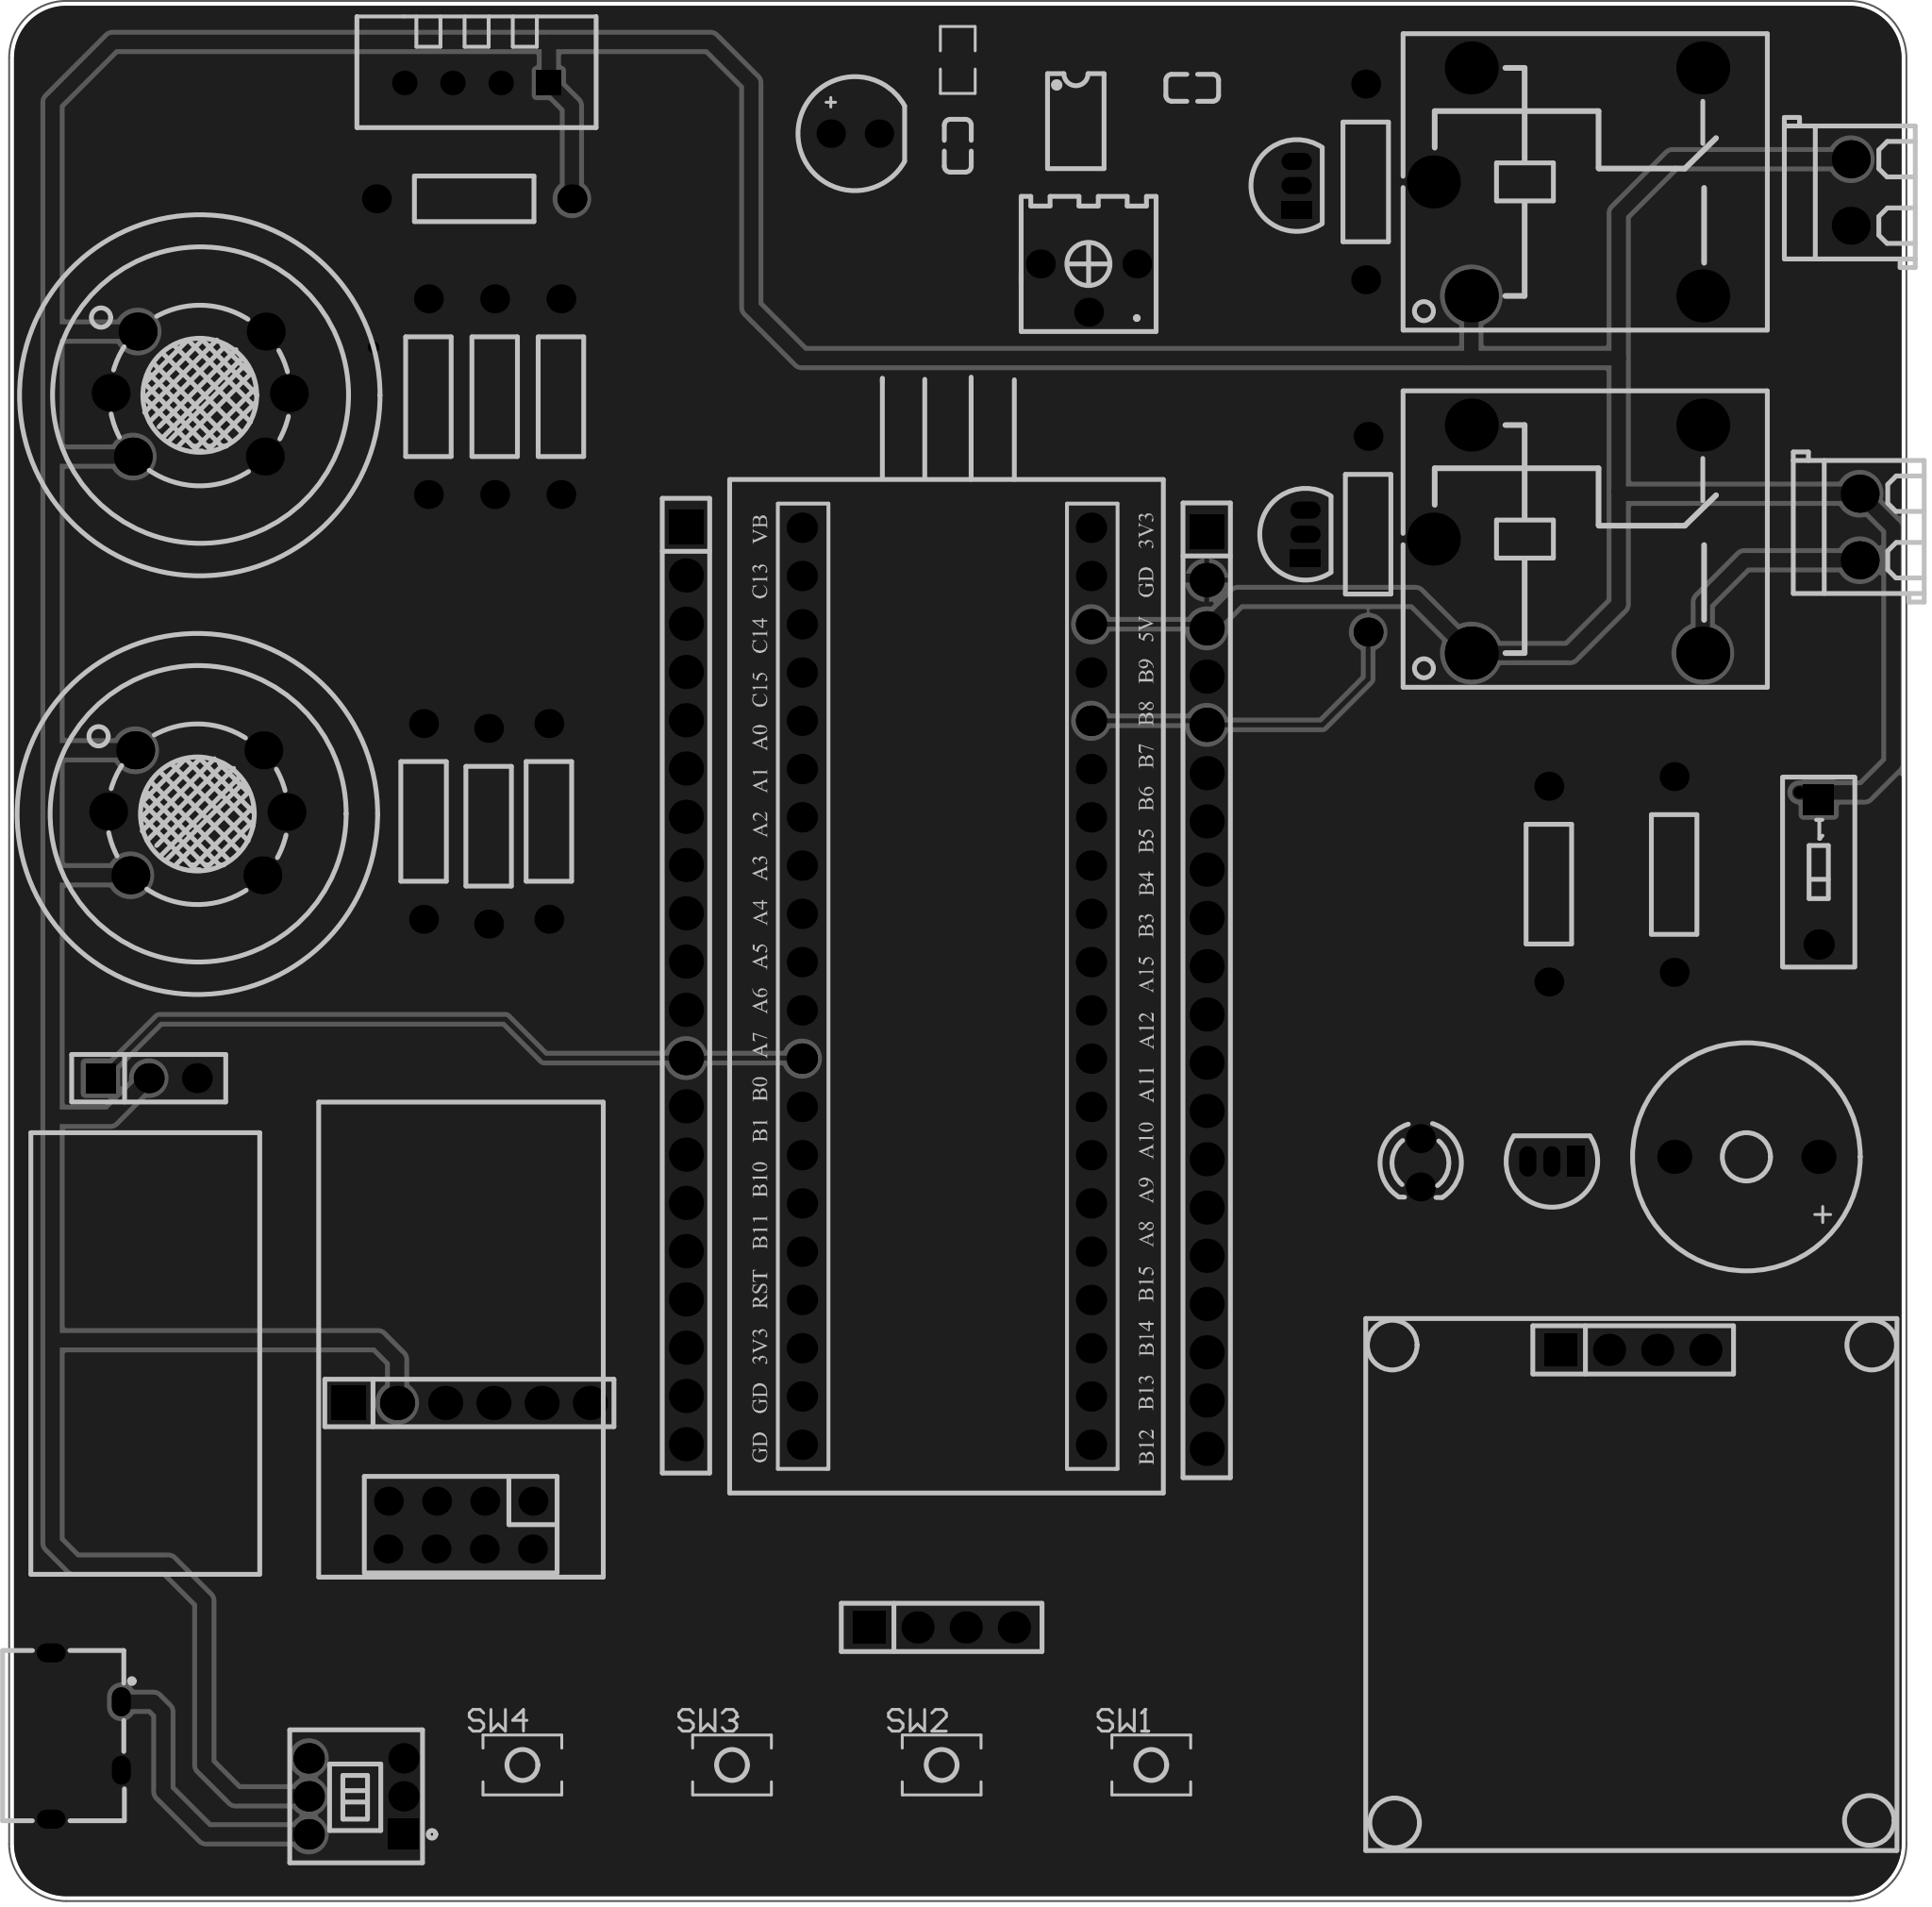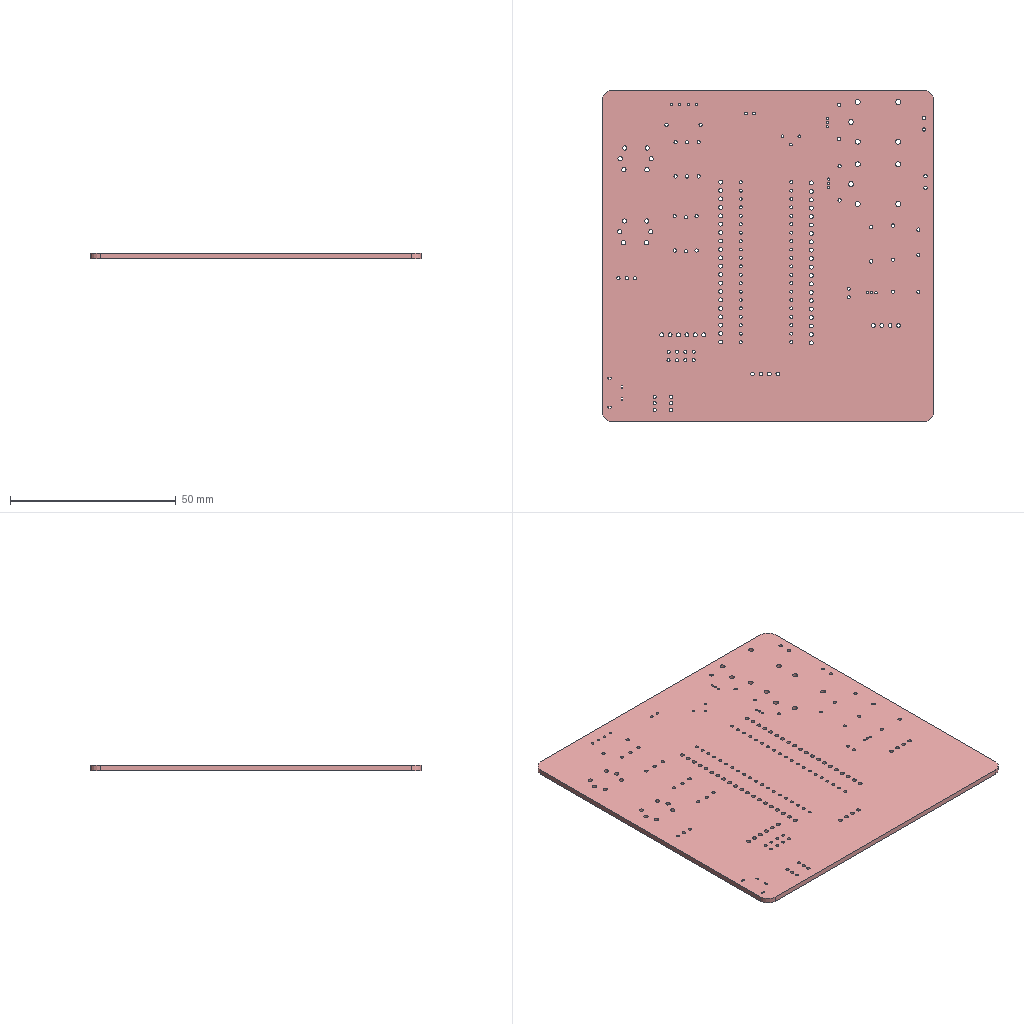Circuit board layout | Altium Designer | box 100 x 100 x 1.6 mm
Layer stack:
# Altium Designer layer stack of  (unit mm; dielectric type: 0 none, 1 core, 2 prepreg, 3 surface material)
index,name,kind,layer,copper_thickness_mm,dielectric_type,dielectric_thickness_mm,dielectric_material,dielectric_constant
0,Top Paste Mask Layer,other,,,,,,
1,Top Silkscreen Layer,other,,,,,,
2,Top Solder Mask Layer,dielectric,,,3,0.01,,3.3
3,Top Layer,copper,Top Layer,0.035,,,,
4,Dielectric1,dielectric,,,3,1.51,FR4,4.5
5,Bottom Layer,copper,Bottom Layer,0.035,,,,
6,Bottom Solder Mask Layer,dielectric,,,3,0.01,,3.3
7,Bottom Silkscreen Layer,other,,,,,,
8,Bottom Paste Mask Layer,other,,,,,,
# drill layer pairs: low layer,high layer
drill_pair,Top Layer,Bottom Layer
Part placement:
Designator,Comment,Layer,Footprint,Center-X(mm),Center-Y(mm),Rotation
H3,,TopLayer,HDR-TH_20P-P2.54-V-F,146.812,132.588,270
H4,,TopLayer,HDR-TH_20P-P2.54-V-F,119.366,132.831,270
H6,,TopLayer,HDR-TH_3P-P2.54-V-F,91.048,127.962,0
H7,,TopLayer,HDR-TH_4P-P2.54-V-F,132.842,99.06,0
SW5,NDS-01V,TopLayer,SW-TH_2P-L3.9-W9.9-P2.54-LS7.6,179.07,138.811,270
U1,MQ-2,TopLayer,SENSOR-TH_MQ-2,93.614,141.932,0
U7,DHT11,TopLayer,SENSOR-TH_DHT11,108.331,180.34,180
BUZZER1,2.3kHz,TopLayer,BUZ-TH_BD12.0-P7.60-D0.6-FD,175.26,123.825,180
H10,2.54-1*4P female,TopLayer,HDR-TH_4P-P2.54-V-F,169.291,113.665,0
H13,,TopLayer,HDR-TH_6P-P2.54-V-M-1,107.95,110.871,0
Q1,,TopLayer,S8050_TO_92,165.006,123.586,180
R8,1kΩ,TopLayer,Res_1/4W,171.45,138.684,270
R9,120,TopLayer,Res_1/4W,164.846,138.176,270
SW8,TK-6700-1,TopLayer,SW-TH_TK-6700-1,101.981,90.17,90
U2,MQ-5,TopLayer,SENSOR-TH_MQ-2,93.741,163.967,0
U44,,TopLayer,STM32最小系统板,133.098,132.803,0
U98,,TopLayer,WiFi封装,107.479,104.445,0
USB1,KH-TYPE-C-2P,TopLayer,USB-SMD_KH-TYPE-C-2P,87.757,93.345,270
Q2,,TopLayer,S8050_TO_92,151.556,174.944,90
R1,10kΩ,TopLayer,Res_1/4W,108.966,141.224,90
R2,10kΩ,TopLayer,Res_1/4W,112.141,141.478,90
R3,5Ω,TopLayer,Res_1/4W,105.537,141.478,90
R4,10kΩ,TopLayer,Res_1/4W,109.284,163.83,90
R5,10kΩ,TopLayer,Res_1/4W,112.776,163.83,90
R6,5Ω,TopLayer,Res_1/4W,105.791,163.83,90
R13,10kΩ,TopLayer,Res_1/4W,108.204,174.244,0
R15,1kΩ,TopLayer,Res_1/4W,155.194,175.133,90
RLY1,SRD-05VDC-SL-C,TopLayer,RELAY-TH_SRD-XXVDC-XL-C,165.862,175.133,0
U4,KF350-3.5-2P,TopLayer,CONN-TH_P3.50_KF350-3.5-2P,180.759,174.577,90
Q3,,TopLayer,S8050_TO_92,152.019,156.591,90
R10,1kΩ,TopLayer,Res_1/4W,155.321,156.591,90
RLY2,SRD-05VDC-SL-C,TopLayer,RELAY-TH_SRD-XXVDC-XL-C,165.862,156.337,0
U5,KF350-3.5-2P,TopLayer,CONN-TH_P3.50_KF350-3.5-2P,181.229,156.972,90
LED1,,TopLayer,LED_TH-3mm,158.077,123.513,270
C1,100nF,TopLayer,C0603,146.05,180.086,180
C2,100nF,TopLayer,C0603,133.693,177.038,90
D1,IR receiver,TopLayer,IR_½ÓÊÕ_D5,128.27,177.673,0
R7,-,TopLayer,RES-ADJ-TH_3362P,140.589,169.545,180
R11,10K,TopLayer,R0805,133.692,181.551,90
SW1,,TopLayer,Key_SMD_3x4x2,143.891,91.821,0
SW2,,TopLayer,Key_SMD_3x4x2,132.842,91.821,0
SW3,,TopLayer,Key_SMD_3x4x2,121.793,91.821,0
SW4,,TopLayer,Key_SMD_3x4x2,110.744,91.821,0
U3,LM393,TopLayer,SOP-8_L4.9-W3.9-P1.27-LS6.0-BL,139.921,178.332,270
Pad and via stacks:
# Altium Designer via and pad stacks of  (unit mm). Each distinct definition once, with the count of objects using it.
# via: kind,start_layer,end_layer,hole_mm,diameter_mm,mode(0 simple;1 top-mid-bottom;2 full stack),diameter_per_layer,count,example_net
# pad: kind,layer,hole_mm,hole_type(0 round;1 square;2 slot),plating,top_size,top_shape(1 round;2 rect;3 octagon;9 rounded rect),mid_size,bottom_size,mode,footprint,size_per_layer,count,example
pad,Multi-Layer,1.2,0,plated,1.8x1.8,2,1.8x1.8,1.8x1.8,0,HDR-TH_20P-P2.54-V-F,,2,H3.1
pad,Multi-Layer,1.2,0,plated,1.8x1.8,1,1.8x1.8,1.8x1.8,0,HDR-TH_20P-P2.54-V-F,,38,H3.2
pad,Multi-Layer,1.02,0,plated,1.575x1.575,1,1.575x1.575,1.575x1.575,0,HDR-TH_3P-P2.54-V-F,,2,H6.3
pad,Multi-Layer,1.02,0,plated,1.575x1.575,2,1.575x1.575,1.575x1.575,0,HDR-TH_3P-P2.54-V-F,,1,H6.1
pad,Multi-Layer,1.1,0,plated,1.7x1.7,2,1.7x1.7,1.7x1.7,0,HDR-TH_4P-P2.54-V-F,,2,H7.1
pad,Multi-Layer,1.1,0,plated,1.7x1.7,1,1.7x1.7,1.7x1.7,0,HDR-TH_4P-P2.54-V-F,,6,H7.2
pad,Multi-Layer,1,0,plated,1.6x1.6,2,1.6x1.6,1.6x1.6,0,SW-TH_2P-L3.9-W9.9-P2.54-LS7.6,,1,SW5.1
pad,Multi-Layer,1,0,plated,1.6x1.6,1,1.6x1.6,1.6x1.6,0,SW-TH_2P-L3.9-W9.9-P2.54-LS7.6,,1,SW5.2
pad,Multi-Layer,1.3,0,plated,2x2,1,2x2,2x2,0,SENSOR-TH_MQ-2,,12,U1.1
pad,Multi-Layer,0.7112,0,plated,1.295x1.295,2,1.295x1.295,1.295x1.295,0,SENSOR-TH_DHT11,,1,U7.1
pad,Multi-Layer,0.7112,0,plated,1.295x1.295,1,1.295x1.295,1.295x1.295,0,SENSOR-TH_DHT11,,3,U7.2
pad,Multi-Layer,1,0,plated,1.8x1.8,1,1.8x1.8,1.8x1.8,0,BUZ-TH_BD12.0-P7.60-D0.6-FD,,2,BUZZER1.2
pad,Multi-Layer,1.2,0,plated,1.8x1.8,1,1.8x1.8,1.8x1.8,0,HDR-TH_6P-P2.54-V-M-1,,5,H13.6
pad,Multi-Layer,1.2,0,plated,1.8x1.8,2,1.8x1.8,1.8x1.8,0,HDR-TH_6P-P2.54-V-M-1,,1,H13.1
pad,Multi-Layer,0.701,0,plated,0.8992x1.6,2,0.8992x1.6,0.8992x1.6,0,S8050_TO_92,,3,Q1.1
pad,Multi-Layer,0.701,0,plated,0.8992x1.6,1,0.8992x1.6,0.8992x1.6,0,S8050_TO_92,,6,Q1.2
pad,Multi-Layer,1,0,plated,1.524x1.524,1,1.524x1.524,1.524x1.524,0,Res_1/4W,,22,R8.1
pad,Multi-Layer,1,0,plated,1.6x1.6,2,1.6x1.6,1.6x1.6,0,SW-TH_TK-6700-1,,1,SW8.1
pad,Multi-Layer,1,0,plated,1.6x1.6,1,1.6x1.6,1.6x1.6,0,SW-TH_TK-6700-1,,5,SW8.2
pad,Multi-Layer,0.9,0,plated,1.6x1.6,1,1.6x1.6,1.6x1.6,0,STM32\u00D7\u00EE\u00D0\u00A1\u00CF\u00B5\u00CD\u00B3\u00B0\u00E5,,40,U44.40
pad,Multi-Layer,0.9144,0,plated,1.524x1.524,1,1.524x1.524,1.524x1.524,0,WiFi\u00B7\u00E2\u00D7\u00B0,,8,U98.1
pad,Multi-Layer,0.45,2,plated,1x1.524,1,1x1.524,1x1.524,0,USB-SMD_KH-TYPE-C-2P,,2,USB1.1
pad,Multi-Layer,0.5,2,plated,1x1.524,1,1x1.524,1x1.524,0,USB-SMD_KH-TYPE-C-2P,,2,USB1.3
pad,Multi-Layer,1.524,0,plated,2.794x2.794,1,2.794x2.794,2.794x2.794,0,RELAY-TH_SRD-XXVDC-XL-C,,10,RLY1.2
pad,Multi-Layer,1,0,plated,2x2,1,2x2,2x2,0,CONN-TH_P3.50_KF350-3.5-2P,,4,U4.1
pad,Multi-Layer,0.9144,0,plated,1.524x1.524,1,1.524x1.524,1.524x1.524,0,LED_TH-3mm,,2,LED1.1
pad,Multi-Layer,0.9,0,plated,1.5x1.5,1,1.5x1.5,1.5x1.5,0,IR \u00BD\u00D3\u00CA\u00D5 D5,,2,D1.2
pad,Multi-Layer,0.762,0,plated,1.524x1.524,1,1.524x1.524,1.524x1.524,0,RES-ADJ-TH_3362P,,3,R7.3
pad,Top Layer,0,0,plated,0.8x0.9,2,0.8x0.9,0.8x0.9,0,C0603,,4,C1.2
pad,Top Layer,0,0,plated,1.133x1.377,2,1.133x1.377,1.133x1.377,0,R0805,,2,R11.2
pad,Top Layer,0,0,plated,1.53x1.36,2,1.53x1.36,1.53x1.36,0,Key_SMD_3x4x2,,8,SW1.1
pad,Top Layer,0,0,plated,0.63x1.865,1,0.63x1.865,0.63x1.865,0,SOP-8_L4.9-W3.9-P1.27-LS6.0-BL,,8,U3.1
via,Top Layer,Bottom Layer,0.3048,0.61,0,,2,+5V
Copper pours:
name,layer,net,type(0 solid;1 hatched;2 none)
Bottom Layer-GND,Bottom Layer,GND,0
Top Layer-GND,Top Layer,GND,0
Design rules, without the lines most boards share:
# Altium Designer design rules of  (exported by Altium Designer, unit mm)
# columns: name | kind | enabled | priority | scope1 | scope2 | descriptor | typed fields (field=value)
creepage | 65 | enabled | 1 | All | All | Creepage Distance Constraint =(0mil) (All),(All) |